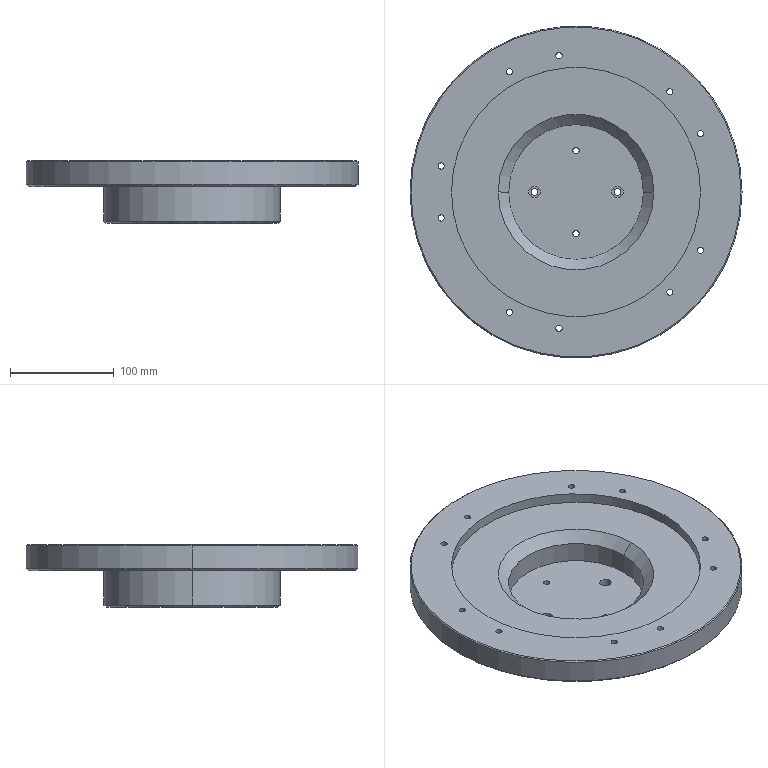NC program | NX | posted with a generic post | part box 320 x 320 x 60 mm
Whole program, first 1569 of 1671 lines:
N10 G17 G21 G94 G90
(FLOOR_WALL_COPY , TOOL : D63)
N12 T01 M6
N14 G54
N16 G17 G0 G90 X-111.041 Y159.693 S6500 M3
N18 G43 Z90. H1
N20 Z63.
N22 G94 G1 Z60. F1250.
N24 X-105.694
N26 X105.696
N28 G2 X107.445 Y158.522 R190.772
N30 X130.313 Y140.326 R191.108
N32 X140.391 Y130.245 R190.747
N34 G1 X-140.394
N36 G3 X-162.829 Y100.796 R191.779
N38 G1 X162.826
N40 G2 X167.72 Y92.43 R190.962
N42 X177.731 Y71.347 R190.522
N44 G1 X-177.72
N46 G3 X-183.779 Y53.845 R190.905
N48 X-186.87 Y41.898 R190.015
N50 G1 X186.872
N52 G2 X188.81 Y32.007 R190.522
N54 X190.35 Y20.971 R189.034
N56 X191.101 Y12.449 R188.892
N58 G1 X-191.099
N60 G3 X-191.307 Y8.671 R190.737
N62 X-191.49 Y2.519 R188.526
N64 G1 Y-2.51
N66 G3 X-191.197 Y-10.802 R188.526
N68 X-190.749 Y-17. R190.562
N70 G1 X190.747
N72 G2 X185.784 Y-46.449 R190.834
N74 G1 X-185.788
N76 G3 X-182.906 Y-56.723 R189.951
N78 X-175.824 Y-75.898 R189.267
N80 G1 X175.831
N82 G2 X159.935 Y-105.347 R190.688
N84 G1 X-159.939
N86 G3 X-151.393 Y-117.272 R184.254
N88 X-136.041 Y-134.796 R190.237
N90 G1 X136.035
N92 X140.226
N94 Z63.
N96 G0 Z90.
N98 M5
(ADAPTIVE_MILLING_COPY , TOOL : D10)
N100 T10 M6
N102 G54
N104 G17 G0 G90 X-167.699 Y-0.751 S7000 M3
N106 G43 Z90. H10
N108 Z45.55
N110 G94 G1 Z42.55 F1000.
N112 X-165.853 Y-0.587 F3000.
N114 G3 X-165.042 Y-0.039 R1.024
N116 X-164.411 Y2.51 R7.406
N118 X-163.825 Y10.487 R163.055
N120 G2 X-150.497 Y65.517 R166.454
N122 X149.112 Y68.574 R164.131
N124 X155.232 Y53.253 R375.404
N126 X5.158 Y-164.038 R164.075
N128 X-164.091 Y-3.174 R164.099
N130 X-163.571 Y2.902 R89.15
N132 X-162.375 Y17.452 R615.566
N134 X148.074 Y68.824 R163.293
N136 X154.541 Y52.674 R266.724
N138 X153.708 Y-55.15 R162.746
N140 X-163.219 Y-4.469 R163.287
N142 X-162.746 Y3.114 R110.67
N144 X-161.065 Y21.334 R295.166
N146 X146.754 Y69.698 R162.464
N148 X154.76 Y49.432 R213.972
N150 X-162.342 Y-6.156 R-162.463
N152 X-161.926 Y3.131 R104.526
N154 X-159.885 Y23.825 R257.116
N156 X145.894 Y69.574 R161.635
N158 X154.348 Y47.983 R200.371
N160 X-161.472 Y-7.049 R-161.633
N162 X-161.066 Y3.739 R119.448
N164 X-158.608 Y26.597 R227.63
N166 X144.775 Y69.997 R160.804
N168 X153.54 Y47.779 R192.297
N170 X-160.584 Y-8.348 R-160.804
N172 X-160.172 Y4.839 R125.799
N174 X-156.919 Y31.22 R200.569
N176 X143.605 Y70.515 R159.979
N178 X153.583 Y44.81 R180.564
N180 X-159.697 Y-9.353 R-159.981
N182 X-159.351 Y4.834 R124.247
N184 X-156. Y31.604 R197.042
N186 X142.382 Y71.125 R159.155
N188 X153.649 Y41.542 R173.736
N190 X-158.796 Y-10.564 R-159.158
N192 X-158.509 Y5.122 R124.27
N194 X-154.853 Y33.058 R191.618
N196 X141.374 Y71.291 R158.324
N198 X152.838 Y41.359 R170.776
N200 X-157.889 Y-11.681 R-158.33
N202 X-157.725 Y4.506 R120.635
N204 X-153.737 Y34.308 R190.113
N206 X140.631 Y70.925 R157.497
N208 X152.312 Y40.119 R168.32
N210 X-156.982 Y-12.703 R-157.502
N212 X-156.891 Y4.682 R121.373
N214 X-152.761 Y34.866 R186.676
N216 X139.478 Y71.367 R156.669
N218 X152.36 Y36.554 R164.249
N220 X-156.122 Y-13.032 R-156.676
N222 X-155.987 Y5.95 R129.61
N224 X-151.223 Y37.751 R179.901
N226 X138.457 Y71.546 R155.842
N228 X151.43 Y36.874 R163.237
N230 X-155.204 Y-14.064 R-155.849
N232 X-155.129 Y6.514 R131.371
N234 X-150.304 Y38.003 R177.491
N236 X137.477 Y71.64 R155.015
N238 X151.366 Y33.5 R160.38
N240 X-154.294 Y-14.9 R-155.021
N242 X-154.34 Y5.976 R128.82
N244 X-149.386 Y38.251 R175.769
N246 X136.122 Y72.443 R154.188
N248 X151.521 Y28.64 R157.78
N250 X-153.369 Y-15.839 R-154.195
N252 X-153.462 Y6.733 R130.459
N254 X-147.931 Y40.526 R171.747
N256 X135.366 Y72.097 R153.359
N258 X151.352 Y24.843 R156.11
N260 X-152.549 Y-15.685 R-153.366
N262 X-152.662 Y6.489 R132.598
N264 X-147.426 Y39.221 R172.911
N266 X133.711 Y73.427 R152.534
N268 X151.266 Y19.744 R154.619
N270 X-151.65 Y-16.329 R-152.538
N272 X-151.81 Y6.841 R133.168
N274 X-146.026 Y41.196 R169.185
N276 X132.568 Y73.784 R151.708
N278 X150.811 Y16.614 R153.419
N280 X16.645 Y-150.815 R151.712
N282 X-150.714 Y-17.27 R151.712
N284 X-150.99 Y6.795 R133.611
N286 X-144.82 Y42.394 R167.722
N288 X132.102 Y72.914 R150.88
N290 X149.799 Y18.15 R152.701
N292 X18.186 Y-149.807 R150.883
N294 X-149.804 Y-17.912 R150.883
N296 X-150.178 Y6.55 R132.106
N298 X-143.829 Y42.822 R165.771
N300 X131.251 Y72.745 R150.053
N302 X149.429 Y13.82 R151.573
N304 X-148.903 Y-18.453 R150.054
N306 X-149.256 Y7.902 R133.377
N308 X-142.307 Y44.972 R163.428
N310 X130.008 Y73.272 R149.224
N312 X148.504 Y14.759 R150.54
N314 X-148.099 Y-18.196 R149.224
N316 X-148.372 Y8.658 R135.611
N318 X-141.051 Y46.159 R161.194
N320 X128.662 Y73.967 R148.394
N322 X148.33 Y4.924 R149.331
N324 X-147.233 Y-18.434 R148.396
N326 X-147.471 Y9.516 R136.787
N328 X-139.127 Y49.235 R157.854
N330 X128.454 Y72.659 R147.566
N332 X147.576 Y1.762 R148.47
N334 X-146.242 Y-19.659 R147.57
N336 X-146.681 Y9.082 R133.855
N338 X-138.561 Y48.342 R157.466
N340 X127.208 Y73.17 R146.734
N342 X146.738 Y-2.405 R147.566
N344 X-145.4 Y-19.687 R146.74
N346 X-145.821 Y9.453 R134.899
N348 X-136.398 Y51.875 R155.266
N350 X126.608 Y72.546 R145.905
N352 X144.722 Y-18.728 R146.401
N354 X-144.547 Y-19.808 R145.909
N356 X-144.88 Y10.726 R136.408
N358 X-134.347 Y54.816 R152.904
N360 X126.012 Y71.916 R145.076
N362 X142.66 Y-26.512 R145.517
N364 X-143.486 Y-21.406 R145.085
N366 X-144.229 Y8.72 R133.432
N368 X-134.283 Y52.745 R153.39
N370 X125.274 Y71.54 R144.251
N372 X144.149 Y-5.85 R144.911
N374 X-142.554 Y-22.003 R144.252
N376 X-143.479 Y7.718 R131.164
N378 X-133.872 Y51.514 R152.99
N380 X124.635 Y70.981 R143.416
N382 X141.417 Y-24.038 R143.816
N384 X-141.637 Y-22.492 R143.424
N386 X-142.69 Y7.225 R131.376
N388 X-132.699 Y52.251 R152.37
N390 X123.308 Y71.628 R142.592
N392 X138.916 Y-32.279 R142.93
N394 X-140.767 Y-22.673 R142.594
N396 X-141.829 Y7.64 R130.576
N398 X-131.097 Y54.014 R150.685
N400 X123.867 Y68.963 R141.762
N402 X58.9 Y-128.979 R141.815
N404 X-139.898 Y-22.842 R141.745
N406 X-140.954 Y8.266 R130.92
N408 X-130.386 Y53.56 R149.841
N410 X135.63 Y38.293 R140.934
N412 X-138.901 Y-23.787 R-140.929
N414 X-140.089 Y8.705 R130.269
N416 X-128.897 Y54.963 R148.15
N418 X121.302 Y70.123 R140.102
N420 X97.155 Y-100.985 R140.198
N422 X-137.931 Y-24.519 R140.096
N424 X-139.254 Y8.761 R129.645
N426 X-127.384 Y56.373 R146.915
N428 X134.78 Y35.088 R139.275
N430 X-136.885 Y-25.627 R-139.269
N432 X-138.549 Y7.139 R127.671
N434 X-126.819 Y55.595 R146.546
N436 X119.752 Y69.49 R138.445
N438 X102.9 Y-92.661 R138.549
N440 X-136.201 Y-24.752 R138.438
N442 X-137.616 Y8.524 R128.789
N444 X-125.679 Y56.112 R145.18
N446 X118.511 Y69.972 R137.618
N448 X121.463 Y-64.745 R137.808
N450 X-135.412 Y-24.45 R137.613
N452 X-136.675 Y9.826 R129.304
N454 X-123.647 Y58.55 R143.55
N456 X117.931 Y69.313 R136.786
N458 X48.497 Y-127.917 R136.813
N460 X-134.588 Y-24.324 R136.745
N462 X-135.831 Y9.952 R128.843
N464 X-122.337 Y59.361 R142.448
N466 X132.864 Y28.822 R135.959
N468 X-133.572 Y-25.259 R-135.947
N470 X-135.064 Y9.202 R127.5
N472 X-121.755 Y58.659 R141.739
N474 X131.4 Y31.491 R135.124
N476 X-132.72 Y-25.288 R-135.115
N478 X-134.275 Y8.674 R126.823
N480 X-121.246 Y57.795 R140.942
N482 X115.856 Y67.919 R134.289
N484 X26.801 Y-131.602 R134.303
N486 X-132.088 Y-24.114 R134.222
N488 X-133.352 Y9.762 R127.509
N490 X-119.639 Y59.202 R139.65
N492 X131.765 Y21.21 R133.468
N494 X-130.954 Y-25.67 R133.453
N496 X-132.589 Y8.981 R126.236
N498 X-119.158 Y58.292 R139.017
N500 X131.636 Y16.232 R132.64
N502 X-130.055 Y-25.922 R132.621
N504 X-131.643 Y10.217 R125.697
N506 X-116.072 Y62.479 R137.001
N508 X130.937 Y15.086 R131.81
N510 X-129.022 Y-26.834 R131.792
N512 X-130.84 Y9.886 R124.887
N514 X-115.395 Y61.976 R136.059
N516 X130.548 Y10.528 R130.976
N518 X-128.172 Y-26.838 R130.96
N520 X-129.972 Y10.278 R124.381
N522 X-114.565 Y61.762 R135.24
N524 X129.689 Y10.818 R130.145
N526 X-127.202 Y-27.4 R130.128
N528 X-129.127 Y10.4 R123.38
N530 X-114.519 Y60.071 R134.471
N532 X110.868 Y66.543 R129.289
N534 X-126.125 Y-28.422 R-129.301
N536 X-128.296 Y10.352 R122.307
N538 X-112.576 Y61.935 R133.333
N540 X109.385 Y67.383 R128.46
N542 X-124.955 Y-29.802 R-128.471
N544 X-127.502 Y9.935 R121.374
N546 X-111.702 Y61.797 R132.559
N548 X126.904 Y13.705 R127.648
N550 X-124.655 Y-27.348 R127.629
N552 X-126.549 Y11.142 R121.707
N554 X-110.664 Y61.946 R131.438
N556 X-86.859 Y-92.405 R-126.816
N558 X-124.847 Y-21.899 R125.96
N560 X-125.312 Y14.565 R123.829
N562 X-105.34 Y69.125 R129.411
N564 X125.656 Y9.031 R125.99
N566 X-122.691 Y-28.486 R125.965
N568 X-124.955 Y10.374 R119.727
N570 X-108.78 Y61.898 R129.761
N572 X124.767 Y9.729 R125.152
N574 X-121.421 Y-30.217 R125.133
N576 X-124.178 Y9.794 R118.71
N578 X-108.621 Y60.482 R129.203
N580 X-96.203 Y-78.746 R-124.318
N582 X-122.555 Y-20.363 R122.928
N584 X-122.585 Y16.101 R122.421
N586 X-99.068 Y73.738 R126.25
N588 X112.961 Y-49.896 R123.496
N590 X-120.048 Y-28.808 R123.465
N592 X-122.326 Y11.527 R118.048
N594 X-105.524 Y62.52 R126.853
N596 X-97.62 Y-74.257 R-122.65
N598 X-121.033 Y-19.257 R121.041
N600 X-120.555 Y18.389 R122.195
N602 X-96.169 Y74.799 R124.293
N604 X107.09 Y58.025 R121.79
N606 X-118.022 Y-30.07 R-121.799
N608 X-120.679 Y11.322 R116.586
N610 X-103.379 Y62.859 R125.301
N612 X120.774 Y7.09 R120.989
N614 X-117.136 Y-30.155 R120.966
N616 X-120.008 Y9.738 R115.469
N618 X-103.66 Y60.763 R124.972
N620 X-93.278 Y-75.734 R-120.149
N622 X-118.217 Y-21.008 R118.896
N624 X-118.303 Y16.632 R118.43
N626 X-94.081 Y73.4 R121.815
N628 X119.035 Y8.088 R119.322
N630 X-115.792 Y-28.651 R119.294
N632 X-118.175 Y11.272 R114.76
N634 X-101.076 Y61.83 R122.839
N636 X103.939 Y56.837 R118.452
N638 X-114.895 Y-28.805 R-118.461
N640 X-117.2 Y12.402 R114.11
N642 X-97.28 Y66.182 R121.253
N644 X106.814 Y49.249 R117.615
N646 X-114.028 Y-28.815 R-117.62
N648 X-116.41 Y11.989 R113.184
N650 X-95.976 Y66.605 R120.37
N652 X103.797 Y53.531 R116.779
N654 X-113.103 Y-29.071 R-116.787
N656 X-115.578 Y11.922 R112.303
N658 X-95.833 Y65.337 R119.566
N660 X-81.851 Y-82.168 R-115.976
N662 X-113.571 Y-23.133 R115.104
N664 X-114.297 Y15.274 R113.391
N666 X-92.904 Y68.036 R118.201
N668 X-80.314 Y-82.505 R-115.14
N670 X-112.728 Y-23.1 R114.301
N672 X-113.201 Y16.886 R113.109
N674 X-91.057 Y69.113 R116.927
N676 X-76.755 Y-84.703 R-114.305
N678 X-111.869 Y-23.114 R113.525
N680 X-112.26 Y17.46 R112.295
N682 X-87.008 Y72.848 R115.55
N684 X-83.119 Y-77.241 R-113.467
N686 X-111.382 Y-21.21 R112.395
N688 X-110.874 Y20.447 R112.816
N690 X-81.695 Y77.548 R114.176
N692 X-73.709 Y-85.167 R-112.632
N694 X-109.942 Y-24.159 R111.895
N696 X-110.915 Y15.314 R110.087
N698 X-89.159 Y67.469 R114.601
N700 X-64.531 Y-91.299 R-111.798
N702 X-108.968 Y-24.696 R111.234
N704 X-110.081 Y15.262 R109.255
N706 X-90.099 Y64.781 R113.906
N708 X110.687 Y7.716 R110.97
N710 X-106.92 Y-29.544 R110.938
N712 X-109.424 Y13.979 R107.582
N714 X-90.271 Y63.089 R113.317
N716 X110.084 Y-2.91 R110.133
N718 X-106.147 Y-29.188 R110.1
N720 X-108.601 Y13.844 R106.889
N722 X-89.081 Y63.322 R112.36
N724 X109.235 Y3.296 R109.295
N726 X-104.989 Y-30.219 R109.264
N728 X-107.917 Y12.678 R105.721
N730 X-88.084 Y63.278 R111.592
N732 X-61.265 Y-89.493 R-108.45
N734 X-105.35 Y-25.485 R107.983
N736 X-106.856 Y14.249 R106.097
N738 X-86.46 Y64.09 R110.587
N740 X-52.586 Y-93.9 R-107.615
N742 X-104.455 Y-25.628 R107.241
N744 X-105.642 Y16.569 R105.729
N746 X-82.974 Y67.209 R109.04
N748 X-59.606 Y-88.598 R-106.774
N750 X-103.665 Y-25.318 R106.349
N752 X-104.618 Y17.567 R105.124
N754 X-79.757 Y69.73 R107.839
N756 X-49.854 Y-93.486 R-105.937
N758 X-102.914 Y-24.846 R105.573
N760 X-103.589 Y18.531 R104.57
N762 X-75.963 Y72.633 R106.656
N764 X-47.1 Y-93.966 R-105.098
N766 X-101.97 Y-25.181 R104.77
N768 X-102.877 Y17.794 R103.577
N770 X-76.461 Y70.882 R105.957
N772 X102.976 Y16.226 R104.26
N774 X-100.524 Y-27.483 R104.228
N776 X-102.304 Y16.239 R102.27
N778 X-78.083 Y67.816 R105.391
N780 X-53.998 Y-88.21 R-103.418
N782 X-100.475 Y-24.186 R102.939
N784 X-101.121 Y18.102 R102.307
N786 X-73.11 Y71.959 R104.195
N788 X-48.01 Y-90.661 R-102.58
N790 X-99.583 Y-24.311 R102.199
N792 X-100.349 Y17.676 R101.415
N794 X-72.075 Y71.811 R103.407
N796 X-55.654 Y-85.176 R-101.739
N798 X-98.886 Y-23.581 R101.192
N800 X-99.215 Y19.092 R100.855
N802 X-62.521 Y79.196 R102.064
N804 X100.87 Y2.216 R100.905
N806 X-96.575 Y-29.065 R100.869
N808 X-99.102 Y15.083 R98.704
N810 X-71.248 Y70.262 R101.899
N812 X-50.538 Y-86.37 R-100.06
N814 X-96.809 Y-25.002 R99.624
N816 X-97.576 Y18.726 R98.775
N818 X-60.892 Y78.338 R100.338
N820 X-53.87 Y-83.328 R-99.217
N822 X-96.107 Y-24.327 R98.682
N824 X-96.326 Y20.573 R98.457
N826 X-51.114 Y84.059 R99.199
N828 X-62.862 Y-75.672 R-98.374
N830 X-95.692 Y-22.4 R97.478
N832 X-95.295 Y21.327 R98.075
N834 X-49.098 Y84.28 R98.323
N836 X-56.725 Y-79.347 R-97.535
N838 X-94.614 Y-23.309 R96.839
N840 X-94.983 Y18.847 R96.598
N842 X-55.952 Y78.865 R97.791
N844 X96.04 Y-11.23 R96.705
N846 X-91.688 Y-30.562 R96.662
N848 X-94.897 Y14.772 R94.242
N850 X-61.287 Y73.707 R97.395
N852 X95.373 Y-9.539 R95.861
N854 X-90.849 Y-30.413 R95.818
N856 X-94.069 Y14.621 R93.509
N858 X-62.509 Y71.559 R96.603
N860 X-63.024 Y-71.09 R-95.006
N862 X-92.705 Y-20.227 R93.851
N864 X-91.427 Y22.974 R95.304
N866 X-42.013 Y84.277 R94.808
N868 X-68.919 Y-64.148 R-94.158
N870 X-92.66 Y-15.754 R92.265
N872 X-84.258 Y40.171 R96.145
N874 X-57.108 Y-73.813 R-93.326
N876 X-90.469 Y-22.474 R92.545
N878 X-90.345 Y20.338 R92.906
N880 X-49.225 Y78.292 R93.383
N882 X-73.322 Y-56.339 R-92.472
N884 X-91.006 Y12.431 R89.768
N886 X-62.032 Y67.458 R93.416
N888 X-64.669 Y-64.906 R-91.63
N890 X-89.879 Y-16.984 R89.903
N892 X-84.765 Y32.634 R92.826
N894 X74.357 Y52.074 R90.82
N896 X-83.379 Y-35.854 R-90.773
N898 X-89.241 Y12.84 R88.343
N900 X-87.005 Y23.41 R128.754
N902 G1 X-85.295 Y29.028
N904 X-85.284 Y29.061
N906 X-83.21 Y34.555
N908 X-83.196 Y34.587
N910 X-80.766 Y39.934
N912 X-80.751 Y39.964
N914 X-77.976 Y45.14
N916 X-77.959 Y45.17
N918 X-74.851 Y50.153
N920 X-74.831 Y50.181
N922 X-71.403 Y54.95
N924 X-71.382 Y54.977
N926 X-67.649 Y59.511
N928 X-67.626 Y59.537
N930 X-63.604 Y63.816
N932 X-63.58 Y63.84
N934 X-59.285 Y67.846
N936 X-59.26 Y67.869
N938 X-54.712 Y71.586
N940 X-54.685 Y71.606
N942 X-49.904 Y75.017
N944 X-49.875 Y75.036
N946 X-44.881 Y78.126
N948 X-44.851 Y78.143
N950 X-39.665 Y80.899
N952 X-39.634 Y80.914
N954 X-34.278 Y83.324
N956 X-34.246 Y83.337
N958 X-28.744 Y85.391
N960 X-28.712 Y85.402
N962 X-23.087 Y87.091
N964 X-23.054 Y87.1
N966 X-17.331 Y88.417
N968 X-17.297 Y88.424
N970 X-11.499 Y89.363
N972 X-11.465 Y89.367
N974 X-5.619 Y89.924
N976 X-5.585 Y89.926
N978 X0.301 Y90.099
N980 X6.189 Y89.887
N982 X6.223 Y89.884
N984 X12.066 Y89.288
N986 X12.1 Y89.283
N988 X17.864 Y88.311
N990 X17.898 Y88.304
N992 X23.586 Y86.958
N994 X23.619 Y86.949
N996 X29.207 Y85.234
N998 X29.24 Y85.223
N1000 X34.704 Y83.148
N1002 X34.736 Y83.134
N1004 X40.054 Y80.707
N1006 X40.084 Y80.692
N1008 X45.232 Y77.923
N1010 X45.262 Y77.905
N1012 X50.219 Y74.806
N1014 X50.247 Y74.787
N1016 X54.991 Y71.372
N1018 X55.018 Y71.351
N1020 X59.529 Y67.633
N1022 X59.554 Y67.61
N1024 X63.813 Y63.606
N1026 X63.837 Y63.582
N1028 X67.826 Y59.309
N1030 X67.849 Y59.283
N1032 X71.55 Y54.759
N1034 X71.571 Y54.732
N1036 X74.969 Y49.975
N1038 X74.988 Y49.947
N1040 X78.069 Y44.979
N1042 X78.086 Y44.95
N1044 X80.837 Y39.791
N1046 X80.852 Y39.761
N1048 X83.26 Y34.434
N1050 X83.273 Y34.403
N1052 X85.328 Y28.93
N1054 X85.339 Y28.898
N1056 X87.034 Y23.303
N1058 X87.043 Y23.27
N1060 X88.368 Y17.577
N1062 X88.375 Y17.544
N1064 X89.327 Y11.776
N1066 X89.331 Y11.742
N1068 X89.904 Y5.925
N1070 X89.907 Y5.891
N1072 X90.1 Y0.031
N1074 X89.928 Y-5.563
N1076 X89.926 Y-5.596
N1078 X89.407 Y-11.152
N1080 X89.403 Y-11.184
N1082 X88.539 Y-16.697
N1084 X88.533 Y-16.729
N1086 X87.327 Y-22.178
N1088 X87.319 Y-22.21
N1090 X85.777 Y-27.573
N1092 X85.767 Y-27.604
N1094 X83.894 Y-32.86
N1096 X83.882 Y-32.891
N1098 X81.685 Y-38.02
N1100 X81.671 Y-38.05
N1102 X79.159 Y-43.033
N1104 X79.143 Y-43.062
N1106 X76.326 Y-47.878
N1108 X76.308 Y-47.906
N1110 X73.034 Y-52.763
N1112 X73.014 Y-52.791
N1114 X69.429 Y-57.424
N1116 X69.408 Y-57.45
N1118 X65.528 Y-61.838
N1120 X65.505 Y-61.863
N1122 X61.347 Y-65.988
N1124 X61.322 Y-66.012
N1126 X56.903 Y-69.856
N1128 X56.877 Y-69.878
N1130 X52.216 Y-73.426
N1132 X52.188 Y-73.446
N1134 X47.306 Y-76.681
N1136 X47.277 Y-76.699
N1138 X42.194 Y-79.609
N1140 X42.164 Y-79.625
N1142 X36.901 Y-82.196
N1144 X36.87 Y-82.21
N1146 X31.451 Y-84.432
N1148 X31.418 Y-84.444
N1150 X25.866 Y-86.307
N1152 X25.833 Y-86.317
N1154 X20.17 Y-87.813
N1156 X20.136 Y-87.82
N1158 X14.388 Y-88.943
N1160 X14.354 Y-88.949
N1162 X8.545 Y-89.693
N1164 X8.511 Y-89.697
N1166 X2.664 Y-90.06
N1168 X2.633 Y-90.061
N1170 X-3.226 Y-90.042
N1172 X-3.261 Y-90.04
N1174 X-9.104 Y-89.638
N1176 X-9.138 Y-89.635
N1178 X-14.943 Y-88.852
N1180 X-14.976 Y-88.846
N1182 X-20.717 Y-87.685
N1184 X-20.751 Y-87.677
N1186 X-26.403 Y-86.144
N1188 X-26.436 Y-86.134
N1190 X-31.977 Y-84.234
N1192 X-32.009 Y-84.222
N1194 X-37.413 Y-81.964
N1196 X-37.444 Y-81.95
N1198 X-42.69 Y-79.344
N1200 X-42.72 Y-79.328
N1202 X-47.784 Y-76.385
N1204 X-47.813 Y-76.367
N1206 X-52.673 Y-73.099
N1208 X-52.701 Y-73.079
N1210 X-57.338 Y-69.5
N1212 X-57.364 Y-69.478
N1214 X-61.757 Y-65.604
N1216 X-61.782 Y-65.581
N1218 X-65.913 Y-61.428
N1220 X-65.936 Y-61.403
N1222 X-69.786 Y-56.989
N1224 X-69.808 Y-56.963
N1226 X-73.361 Y-52.307
N1228 X-73.381 Y-52.279
N1230 X-76.623 Y-47.4
N1232 X-76.641 Y-47.372
N1234 G2 X-81.879 Y-37.6 R105.305
N1236 X-85.878 Y-27.257 R105.312
N1238 X-88.575 Y-16.502 R105.312
N1240 X-89.932 Y-5.497 R105.312
N1242 G1 X-90.1 Y0.03
N1244 X-89.905 Y5.918
N1246 X-89.903 Y5.952
N1248 X-89.324 Y11.797
N1250 X-89.319 Y11.831
N1252 X-88.359 Y17.625
N1254 X-88.352 Y17.658
N1256 X-87.418 Y21.65
N1258 G3 X-88.324 Y22.888 R1.014
N1260 G1 X-89.672 Y22.991
N1262 Z45.55
N1264 G0 Z90.
N1266 X-92.795 Y0.
N1268 Z62.003
N1270 G1 Z59.003 F1000.
N1272 X-91.324 Y-0.459 F3000.
N1274 G3 X-90.148 Y0. R1.017
N1276 X-89.437 Y2.526 R6.856
N1278 G2 X-88.361 Y12.065 R374.925
N1280 X-71.52 Y-53.258 R-89.171
N1282 X-75.508 Y-47.372 R593.008
N1284 X-80.018 Y-39.357 R120.656
N1286 X-89.105 Y-2.561 R87.818
N1288 G3 X-89.138 Y-0.02 R38.159
N1290 G1 X-88.948 Y5.819
N1292 X-88.946 Y5.853
N1294 X-88.373 Y11.65
N1296 X-88.369 Y11.684
N1298 X-87.417 Y17.43
N1300 X-87.411 Y17.464
N1302 X-86.083 Y23.135
N1304 X-86.074 Y23.168
N1306 X-84.378 Y28.74
N1308 X-84.367 Y28.773
N1310 X-82.307 Y34.221
N1312 X-82.294 Y34.253
N1314 X-79.882 Y39.554
N1316 X-79.866 Y39.585
N1318 X-77.111 Y44.716
N1320 X-77.093 Y44.746
N1322 X-74.007 Y49.685
N1324 X-73.987 Y49.714
N1326 X-70.583 Y54.439
N1328 X-70.562 Y54.467
N1330 X-66.854 Y58.959
N1332 X-66.831 Y58.984
N1334 X-62.837 Y63.223
N1336 X-62.812 Y63.247
N1338 X-58.548 Y67.214
N1340 X-58.522 Y67.237
N1342 X-54.006 Y70.915
N1344 X-53.978 Y70.936
N1346 X-49.23 Y74.31
N1348 X-49.202 Y74.329
N1350 X-44.243 Y77.383
N1352 X-44.213 Y77.4
N1354 X-39.063 Y80.123
N1356 X-39.032 Y80.138
N1358 X-33.716 Y82.516
N1360 X-33.684 Y82.529
N1362 X-28.222 Y84.552
N1364 X-28.189 Y84.563
N1366 X-22.607 Y86.224
N1368 X-22.573 Y86.232
N1370 X-16.894 Y87.522
N1372 X-16.86 Y87.529
N1374 X-11.108 Y88.443
N1376 X-11.073 Y88.448
N1378 X-5.274 Y88.982
N1380 X-5.239 Y88.984
N1382 X0.594 Y89.136
N1384 X6.437 Y88.905
N1386 X6.472 Y88.903
N1388 X12.264 Y88.29
N1390 X12.298 Y88.286
N1392 X17.984 Y87.305
N1394 X18.018 Y87.298
N1396 X23.628 Y85.949
N1398 X23.661 Y85.94
N1400 X29.172 Y84.229
N1402 X29.204 Y84.218
N1404 X34.591 Y82.152
N1406 X34.623 Y82.139
N1408 X39.865 Y79.727
N1410 X39.895 Y79.712
N1412 X44.969 Y76.964
N1414 X44.998 Y76.946
N1416 X49.882 Y73.874
N1418 X49.911 Y73.855
N1420 X54.584 Y70.471
N1422 X54.611 Y70.45
N1424 X59.055 Y66.769
N1426 X59.081 Y66.746
N1428 X63.275 Y62.784
N1430 X63.299 Y62.76
N1432 X67.227 Y58.533
N1434 X67.25 Y58.507
N1436 X70.894 Y54.033
N1438 X70.915 Y54.006
N1440 X74.26 Y49.305
N1442 X74.279 Y49.277
N1444 X77.312 Y44.368
N1446 X77.329 Y44.338
N1448 X80.035 Y39.242
N1450 X80.05 Y39.211
N1452 X82.42 Y33.95
N1454 X82.433 Y33.918
N1456 X84.454 Y28.514
N1458 X84.465 Y28.482
N1460 X86.131 Y22.957
N1462 X86.14 Y22.924
N1464 X87.442 Y17.303
N1466 X87.449 Y17.269
N1468 X88.383 Y11.575
N1470 X88.388 Y11.542
N1472 X88.949 Y5.799
N1474 X88.951 Y5.765
N1476 X89.138 Y-0.02
N1478 X88.965 Y-5.549
N1480 X88.963 Y-5.581
N1482 X88.448 Y-11.073
N1484 X88.444 Y-11.105
N1486 X87.587 Y-16.554
N1488 X87.581 Y-16.586
N1490 X86.388 Y-21.971
N1492 X86.38 Y-22.002
N1494 X84.854 Y-27.303
N1496 X84.844 Y-27.334
N1498 X82.991 Y-32.529
N1500 X82.979 Y-32.559
N1502 X80.806 Y-37.629
N1504 X80.793 Y-37.658
N1506 X78.309 Y-42.583
N1508 X78.293 Y-42.612
N1510 X75.508 Y-47.372
N1512 X75.49 Y-47.4
N1514 X72.262 Y-52.189
N1516 X72.242 Y-52.217
N1518 X68.71 Y-56.785
N1520 X68.688 Y-56.812
N1522 X64.865 Y-61.14
N1524 X64.842 Y-61.165
N1526 X60.745 Y-65.235
N1528 X60.72 Y-65.259
N1530 X56.367 Y-69.053
N1532 X56.34 Y-69.075
N1534 X51.749 Y-72.578
N1536 X51.722 Y-72.598
N1538 X46.912 Y-75.795
N1540 X46.883 Y-75.813
N1542 X41.876 Y-78.689
N1544 X41.846 Y-78.705
N1546 X36.661 Y-81.25
N1548 X36.63 Y-81.264
N1550 X31.291 Y-83.465
N1552 X31.259 Y-83.477
N1554 X25.788 Y-85.326
N1556 X25.756 Y-85.336
N1558 X20.176 Y-86.825
N1560 X20.143 Y-86.832
N1562 X14.478 Y-87.954
N1564 X14.444 Y-87.96
N1566 X8.718 Y-88.711
N1568 X8.684 Y-88.714
N1570 X2.922 Y-89.09
N1572 X2.887 Y-89.091
N1574 X-2.887
N1576 X-2.922 Y-89.09
N1578 X-8.684 Y-88.714
N1580 X-8.718 Y-88.711
N1582 X-14.444 Y-87.96
N1584 X-14.478 Y-87.954
N1586 X-20.143 Y-86.832
N1588 X-20.176 Y-86.825
N1590 X-25.756 Y-85.336
N1592 X-25.788 Y-85.326
N1594 X-31.259 Y-83.477
N1596 X-31.291 Y-83.465
N1598 X-36.63 Y-81.264
N1600 X-36.661 Y-81.25
N1602 X-41.846 Y-78.705
N1604 X-41.876 Y-78.689
N1606 X-46.883 Y-75.813
N1608 X-46.912 Y-75.795
N1610 X-51.722 Y-72.598
N1612 X-51.749 Y-72.578
N1614 X-56.34 Y-69.075
N1616 X-56.367 Y-69.053
N1618 X-60.72 Y-65.259
N1620 X-60.745 Y-65.235
N1622 X-64.842 Y-61.165
N1624 X-64.865 Y-61.14
N1626 X-68.688 Y-56.812
N1628 X-68.71 Y-56.785
N1630 X-72.242 Y-52.217
N1632 X-72.262 Y-52.189
N1634 X-75.49 Y-47.4
N1636 X-75.508 Y-47.372
N1638 X-78.293 Y-42.612
N1640 X-78.309 Y-42.583
N1642 X-80.793 Y-37.658
N1644 X-80.806 Y-37.629
N1646 X-82.979 Y-32.559
N1648 X-82.991 Y-32.529
N1650 X-84.844 Y-27.334
N1652 X-84.854 Y-27.303
N1654 X-86.38 Y-22.002
N1656 X-86.388 Y-21.971
N1658 X-87.581 Y-16.586
N1660 X-87.587 Y-16.554
N1662 X-88.444 Y-11.105
N1664 X-88.448 Y-11.073
N1666 X-88.963 Y-5.581
N1668 X-88.965 Y-5.549
N1670 X-89.078 Y-1.95
N1672 G3 X-90.126 Y-0.973 R1.014
N1674 G1 X-91.457 Y-1.024
N1676 Z62.003
N1678 G0 Z90.
N1680 X-167.7 Y-0.752
N1682 Z28.1
N1684 G1 Z25.1 F1000.
N1686 X-165.854 Y-0.588 F3000.
N1688 G3 X-165.044 Y-0.04 R1.024
N1690 X-164.412 Y2.509 R7.403
N1692 X-163.827 Y10.486 R162.42
N1694 G2 X-152.859 Y59.783 R166.573
N1696 X149.23 Y68.305 R164.119
N1698 X155.166 Y53.448 R410.848
N1700 X-88.126 Y-138.453 R164.103
N1702 X-164.092 Y-3.082 R164.037
N1704 X-163.508 Y3.591 R121.795
N1706 X-162.069 Y20.025 R304.249
N1708 X148.233 Y68.47 R163.282
N1710 X154.672 Y52.309 R260.699
N1712 X61.143 Y-151.418 R163.202
N1714 X-163.223 Y-4.486 R163.274
N1716 X-162.676 Y4.095 R148.592
N1718 X-160.561 Y24.881 R247.607
N1720 X147.205 Y68.718 R162.453
N1722 X154.377 Y50.591 R222.805
N1724 X-162.347 Y-6.084 R-162.46
N1726 X-161.96 Y2.704 R103.55
N1728 X-159.876 Y23.896 R260.095
N1730 X145.964 Y69.42 R161.635
N1732 X154.312 Y48.11 R200.655
N1734 X-161.47 Y-7.188 R-161.636
N1736 X-161.01 Y4.599 R127.931
N1738 X-158.478 Y27.347 R215.632
N1740 X144.841 Y69.853 R160.802
N1742 X153.504 Y47.917 R192.042
N1744 X-160.59 Y-8.297 R-160.809
N1746 X-160.23 Y3.992 R119.696
N1748 X-157.252 Y29.502 R209.569
N1750 X143.449 Y70.831 R159.982
N1752 X153.457 Y45.246 R180.558
N1754 X-159.713 Y-9.114 R-159.983
N1756 X-159.305 Y5.572 R129.984
N1758 X-155.833 Y32.426 R194.499
N1760 X142.659 Y70.552 R159.149
N1762 X153.011 Y43.819 R175.213
N1764 X-158.819 Y-10.238 R-159.158
N1766 X-158.495 Y5.449 R130.394
N1768 X-155.034 Y32.203 R193.738
N1770 X141.473 Y71.091 R158.327
N1772 X153.059 Y40.566 R170.705
N1774 X-157.92 Y-11.268 R-158.334
N1776 X-157.67 Y5.518 R131.532
N1778 X-153.819 Y33.931 R189.514
N1780 X140.321 Y71.541 R157.504
N1782 X152.546 Y39.238 R167.313
N1784 X-157.051 Y-11.804 R-157.504
N1786 X-156.848 Y5.482 R132.678
N1788 X-152.673 Y35.257 R185.868
N1790 X139.067 Y72.169 R156.675
N1792 X152.39 Y36.46 R163.976
N1794 X-156.169 Y-12.443 R-156.679
N1796 X-155.951 Y6.639 R135.158
N1798 X-151.762 Y35.505 R181.537
N1800 X138.543 Y71.378 R155.84
N1802 X151.712 Y35.72 R162.27
N1804 X-155.246 Y-13.587 R-155.852
N1806 X-155.164 Y6.095 R131.411
N1808 X-150.67 Y36.527 R179.505
N1810 X137.468 Y71.659 R155.016
N1812 X151.792 Y31.569 R159.718
N1814 X-154.303 Y-14.833 R-155.028
N1816 X-154.344 Y6.044 R130.68
N1818 X-149.17 Y39.091 R176.325
N1820 X136.573 Y71.589 R154.191
N1822 X151.652 Y27.989 R157.808
N1824 X-153.299 Y-16.58 R-154.204
N1826 X-153.493 Y6.389 R130.3
N1828 X-148.096 Y39.902 R172.595
N1830 X135.346 Y72.139 R153.361
N1832 X151.184 Y25.877 R156.164
N1834 X-152.447 Y-16.738 R-153.374
N1836 X-152.663 Y6.429 R130.176
N1838 X-146.36 Y43.015 R169.183
N1840 X134.159 Y72.6 R152.529
N1842 X150.726 Y23.567 R155.048
N1844 X-151.539 Y-17.395 R-152.546
N1846 X-151.864 Y6.071 R130.207
N1848 X-145.932 Y41.51 R169.421
N1850 X133.204 Y72.621 R151.7
N1852 X150.086 Y22.243 R153.78
N1854 X-150.571 Y-18.55 R-151.718
N1856 X-151.04 Y6.008 R129.542
N1858 X-144.731 Y42.692 R167.689
N1860 X132.963 Y71.325 R150.874
N1862 X149.041 Y23.59 R153.076
N1864 X-149.615 Y-19.506 R-150.889
N1866 X-150.194 Y6.344 R130.112
N1868 X-143.453 Y44.06 R165.526
N1870 X131.583 Y72.14 R150.049
N1872 X148.732 Y19.991 R151.835
N1874 X20.019 Y-148.741 R150.063
N1876 X-148.572 Y-21.054 R150.063
N1878 X-149.379 Y6.184 R129.584
N1880 X-142.812 Y43.325 R164.8
N1882 X130.674 Y72.07 R149.215
N1884 X148.127 Y18.166 R150.632
N1886 X-147.752 Y-20.913 R149.23
N1888 X-148.51 Y6.824 R130.899
N1890 X-141.906 Y43.452 R163.188
N1892 X129.673 Y72.174 R148.39
N1894 X148.035 Y10.559 R149.488
N1896 X-146.792 Y-21.759 R148.403
N1898 X-147.728 Y6.171 R129.922
N1900 X-141.119 Y43.201 R162.978
N1902 X128.326 Y72.882 R147.563
N1904 X147.553 Y2.921 R148.313
N1906 X-145.96 Y-21.71 R147.572
N1908 X-146.827 Y7.218 R130.499
N1910 X-140.062 Y43.814 R161.074
N1912 X127.912 Y71.929 R146.735
N1914 X146.631 Y-6.129 R147.415
N1916 X-144.859 Y-23.432 R146.748
N1918 X-145.98 Y7.474 R130.501
N1920 X-138.966 Y44.527 R159.448
N1922 X127.691 Y70.616 R145.904
N1924 X145.477 Y-11.479 R146.439
N1926 X-143.866 Y-24.355 R145.918
N1928 X-145.201 Y6.84 R130.083
N1930 X-137.391 Y46.669 R158.337
N1932 X126.259 Y71.483 R145.078
N1934 X142.648 Y-26.608 R145.528
N1936 X-142.85 Y-25.368 R145.094
N1938 X-144.388 Y6.613 R129.435
N1940 X-136.335 Y47.2 R157.043
N1942 X125.317 Y71.469 R144.256
N1944 X141.248 Y-29.427 R144.714
N1946 X-142.019 Y-25.287 R144.263
N1948 X-143.543 Y6.892 R129.404
N1950 X-134.934 Y48.679 R155.564
N1952 X124.128 Y71.88 R143.433
N1954 X143.237 Y-7.613 R144.031
N1956 X-141.395 Y-24.016 R143.427
N1958 X-142.611 Y8.278 R130.736
N1960 X-132.973 Y51.56 R152.638
N1962 X124.425 Y69.672 R142.596
N1964 X129.312 Y-60.17 R142.836
N1966 X-140.209 Y-25.984 R142.605
N1968 X-141.728 Y8.877 R130.079
N1970 X-131.197 Y53.776 R150.427
N1972 X123.3 Y69.977 R141.765
N1974 X115.976 Y-81.579 R141.88
N1976 X-139.199 Y-26.853 R141.774
N1978 X-140.905 Y8.792 R129.195
N1980 X-130.488 Y53.309 R149.483
N1982 X135.476 Y38.847 R140.937
N1984 X-138.524 Y-25.937 R-140.935
N1986 X-140.076 Y8.822 R129.303
N1988 X-129.818 Y52.766 R149.255
N1990 X136.214 Y32.814 R140.118
N1992 X-137.483 Y-26.974 R-140.108
N1994 X-139.229 Y9.065 R129.109
N1996 X-128.647 Y53.438 R148.263
N1998 X135.3 Y33.053 R139.286
N2000 X-136.57 Y-27.307 R-139.277
N2002 X-138.418 Y8.825 R128.383
N2004 X-127.886 Y53.106 R147.301
N2006 X119.996 Y69.067 R138.45
N2008 X-134.903 Y-31.142 R-138.453
N2010 X-137.572 Y9. R127.775
N2012 X-125.855 Y55.73 R145.323
N2014 X137.553 Y-4.378 R137.632
N2016 X-135.194 Y-25.662 R137.612
N2018 X-136.61 Y10.49 R129.048
N2020 X-124.377 Y56.98 R143.609
N2022 X117.25 Y70.46 R136.781
N2024 X-134.068 Y-27.118 R-136.79
N2026 X-135.783 Y10.406 R128.01
N2028 X-123.675 Y56.517 R142.554
N2030 X135.157 Y14.761 R135.966
N2032 X-133.306 Y-26.69 R135.955
N2034 X-134.931 Y10.64 R127.807
N2036 X-123.087 Y55.798 R141.695
N2038 X-129.292 Y-39.336 R-135.14
N2040 X-134.16 Y9.999 R126.279
N2042 X-122.287 Y55.556 R141.031
N2044 X-127.511 Y-42.208 R-134.31
N2046 X-133.32 Y10.078 R125.781
N2048 X-120.931 Y56.514 R139.644
N2050 X-110.37 Y-75.076 R-133.479
N2052 X-132.186 Y-17.861 R131.456
N2054 X-131.876 Y15.548 R131.74
N2056 X-112.46 Y70.356 R135.9
N2058 X-107.928 Y-77.126 R-132.649
N2060 X-131.297 Y-18.228 R130.751
N2062 X-131.075 Y15.279 R130.727
N2064 X-111.172 Y70.841 R135.105
N2066 X35.839 Y-126.848 R-131.818
N2068 X-128.627 Y-28.711 R131.768
N2070 X-130.811 Y10.165 R124.065
N2072 X-117.017 Y58.853 R136.2
N2074 X-125.2 Y-38.49 R-130.982
N2076 X-129.998 Y9.948 R123.085
N2078 X-115.655 Y59.701 R135.361
N2080 X-123.669 Y-40.57 R-130.151
N2082 X-129.193 Y9.661 R122.5
N2084 X-115.501 Y58.166 R134.575
N2086 X-123.023 Y-39.856 R-129.317
N2088 X-128.27 Y10.597 R122.046
N2090 X-113.078 Y61.009 R133.071
N2092 X-122.863 Y-37.588 R-128.484
N2094 X-127.495 Y9.97 R121.097
N2096 X-113.566 Y58.297 R132.601
N2098 X-122.053 Y-37.388 R-127.652
N2100 X-126.662 Y9.972 R120.388
N2102 X-113.008 Y57.556 R131.79
N2104 X-121.514 Y-36.296 R-126.818
N2106 X-125.737 Y10.902 R120.088
N2108 X-110.338 Y60.826 R130.675
N2110 X-120.199 Y-37.753 R-125.988
N2112 X-124.86 Y11.269 R119.51
N2114 X-108.532 Y62.33 R129.261
N2116 X-119.265 Y-37.932 R-125.153
N2118 X-124.026 Y11.273 R118.789
N2120 X-106.629 Y63.933 R128.331
N2122 X-108.939 Y-59.901 R-124.321
N2124 X-123.489 Y-12.747 R120.326
N2126 X-120.096 Y28.93 R128.733
N2128 X100.56 Y71.686 R123.542
N2130 X37.934 Y-117.531 R123.53
N2132 X-119.834 Y-29.723 R123.48
N2134 X-122.243 Y12.282 R118.237
N2136 X-104.931 Y63.515 R126.447
N2138 X-116.438 Y-38.545 R-122.653
N2140 X-121.45 Y11.9 R116.843
N2142 X-105.055 Y61.683 R125.884
N2144 X-113.941 Y-43.101 R-121.82
N2146 X-120.706 Y11.06 R115.932
N2148 X-104.488 Y61. R125.253
N2150 X16.762 Y-119.812 R-120.986
N2152 X-117.69 Y-27.896 R120.866
N2154 X-119.627 Y13.142 R116.464
N2156 X-101.834 Y63.777 R123.737
N2158 X-113.578 Y-39.191 R-120.151
N2160 X-118.974 Y11.591 R114.69
N2162 X-102.43 Y61.205 R123.41
N2164 X-110.39 Y-45.277 R-119.316
N2166 X-118.302 Y10.081 R113.747
N2168 X-102.908 Y58.731 R123.105
N2170 X-108.845 Y-46.803 R-118.482
N2172 X-117.376 Y10.903 R113.16
N2174 X-101.401 Y59.666 R121.998
N2176 X-109.015 Y-44.227 R-117.646
N2178 X-116.472 Y11.472 R112.395
N2180 X-98.369 Y63.005 R120.384
N2182 X-109.681 Y-40.184 R-116.811
N2184 X-115.559 Y12.088 R111.795
N2186 X-96.464 Y64.392 R119.199
N2188 X105.961 Y47.088 R115.937
N2190 X-111.975 Y-30.098 R-115.954
N2192 X-114.6 Y13.048 R111.905
N2194 X-93.516 Y67.184 R118.062
N2196 X110.306 Y-33.03 R115.148
N2198 X-110.716 Y-31.52 R115.125
N2200 X-113.847 Y12.373 R110.756
N2202 X-94.81 Y63.853 R117.392
N2204 X-107.889 Y-37.741 R-114.302
N2206 X-113.178 Y10.955 R109.61
N2208 X-95.13 Y61.859 R117.017
N2210 X109.931 Y-28.147 R113.478
N2212 X-109.435 Y-29.874 R113.452
N2214 X-112.29 Y11.377 R109.536
N2216 X-94.589 Y61.157 R116.066
N2218 X109.81 Y-25.084 R112.641
N2220 X-108.161 Y-31.332 R112.62
N2222 X-111.464 Y11.259 R108.617
N2224 X-92.076 Y63.414 R115.073
N2226 X-94.067 Y-60.412 R-111.795
N2228 X-110.775 Y-13.651 R108.529
N2230 X-94.946 Y57.433 R115.101
N2232 X-83.66 Y-72.893 R-110.959
N2234 X-109.072 Y-19.794 R109.372
N2236 X-108.224 Y20.965 R111.145
N2238 X-64.592 Y89.193 R111.077
N2240 X-86.939 Y-67.591 R-110.122
N2242 X-108.653 Y-17.072 R107.982
N2244 X-105.903 Y27.248 R112.13
N2246 X-1.456 Y109.282 R109.509
N2248 X-61.243 Y-90.522 R-109.29
N2250 X-106.207 Y-25.504 R108.741
N2252 X-107.443 Y15.914 R107.176
N2254 X-79.629 Y73.622 R110.269
N2256 X-101.477 Y-38.241 R-108.445
N2258 X-107.373 Y10.243 R104.409
N2260 X-88.458 Y61.288 R110.834
N2262 X-99.152 Y-41.813 R-107.609
N2264 X-106.604 Y9.586 R103.434
N2266 X-88.307 Y60.024 R110.158
N2268 X-84.118 Y-65.756 R-106.771
N2270 X-105.093 Y-18.121 R104.668
N2272 X-103.351 Y23.677 R107.829
N2274 X-40.409 Y97.932 R106.496
N2276 X-78.512 Y-71.119 R-105.935
N2278 X-103.784 Y-20.707 R104.399
N2280 X-102.815 Y22.283 R106.056
N2282 X-51.715 Y91.495 R105.833
N2284 X-97.338 Y-39.621 R-105.094
N2286 X-103.854 Y11.492 R101.354
N2288 X-79.948 Y66.92 R106.711
N2290 X-82.416 Y-63.846 R-104.255
N2292 X-102.756 Y-16.705 R101.853
N2294 X-99.475 Y28.524 R106.198
N2296 X8.012 Y103.115 R103.619
N2298 X-56.119 Y-86.87 R-103.422
N2300 X-100.523 Y-23.986 R102.779
N2302 X-100.768 Y19.873 R102.752
N2304 X-62.474 Y81.36 R103.695
N2306 X-94.731 Y-39.332 R-102.575
N2308 X-101.437 Y10.559 R99.008
N2310 X-77.037 Y66.458 R104.177
N2312 X-80.439 Y-62.285 R-101.736
N2314 X-100.056 Y-17.606 R99.324
N2316 X-97.739 Y25.412 R103.04
N2318 X-22.646 Y98.332 R101.332
N2320 X-77.368 Y-64.763 R-100.898
N2322 X-99.158 Y-17.887 R98.858
N2324 X-96.045 Y28.305 R102.479
N2326 X-2.906 Y100.025 R100.324
N2328 X-85.144 Y-52.546 R-100.056
N2330 X-98.908 Y10.506 R96.609
N2332 X-75.034 Y64.915 R101.474
N2334 X-91.315 Y-38.778 R-99.213
N2336 X-97.802 Y12.467 R95.919
N2338 X-68.441 Y70.671 R100.199
N2340 X-82.052 Y-54.265 R-98.375
N2342 X-96.944 Y12.53 R95.201
N2344 X-65.419 Y72.347 R99.202
N2346 X-81.436 Y-53.667 R-97.532
N2348 X-96.215 Y11.69 R94.411
N2350 X-65.992 Y70.679 R98.498
N2352 X-85.398 Y-45.333 R-96.689
N2354 X-95.493 Y10.742 R93.46
N2356 X-68.117 Y67.437 R97.816
N2358 X-86.802 Y-40.62 R-95.846
N2360 X-94.467 Y12.065 R92.845
N2362 X-65.671 Y68.663 R96.832
N2364 X-84.979 Y-42.459 R-95.003
N2366 X-93.71 Y11.402 R91.956
N2368 X-64.935 Y68.2 R96.038
N2370 X-84.197 Y-42.139 R-94.161
N2372 X-92.816 Y11.728 R91.274
N2374 X-63.982 Y67.94 R95.156
N2376 X-83.813 Y-41.012 R-93.317
N2378 X-91.757 Y13.139 R90.574
N2380 X-61.326 Y69.224 R94.143
N2382 X-83.291 Y-40.15 R-92.473
N2384 X-90.884 Y13.266 R89.833
N2386 X-61.332 Y68.089 R93.333
N2388 X-81.85 Y-41.171 R-91.63
N2390 X-90.21 Y12.113 R88.971
N2392 X-62.858 Y65.514 R92.675
N2394 X-82.293 Y-38.317 R-90.784
N2396 X-89.242 Y12.848 R88.339
N2398 X-87.005 Y23.41 R129.575
N2400 G1 X-85.295 Y29.028
N2402 X-85.284 Y29.061
N2404 X-83.21 Y34.555
N2406 X-83.196 Y34.587
N2408 X-80.766 Y39.934
N2410 X-80.751 Y39.964
N2412 X-77.976 Y45.14
N2414 X-77.959 Y45.17
N2416 X-74.851 Y50.153
N2418 X-74.831 Y50.181
N2420 X-71.403 Y54.95
N2422 X-71.382 Y54.977
N2424 X-67.649 Y59.511
N2426 X-67.626 Y59.537
N2428 X-63.604 Y63.816
N2430 X-63.58 Y63.84
N2432 X-59.285 Y67.846
N2434 X-59.26 Y67.869
N2436 X-54.712 Y71.586
N2438 X-54.685 Y71.606
N2440 X-49.904 Y75.017
N2442 X-49.875 Y75.036
N2444 X-44.881 Y78.126
N2446 X-44.851 Y78.143
N2448 X-39.665 Y80.899
N2450 X-39.634 Y80.914
N2452 X-34.278 Y83.324
N2454 X-34.246 Y83.337
N2456 X-28.744 Y85.391
N2458 X-28.712 Y85.402
N2460 X-23.087 Y87.091
N2462 X-23.054 Y87.1
N2464 X-17.331 Y88.417
N2466 X-17.297 Y88.424
N2468 X-11.499 Y89.363
N2470 X-11.465 Y89.367
N2472 X-5.619 Y89.924
N2474 X-5.585 Y89.926
N2476 X0.301 Y90.099
N2478 X6.189 Y89.887
N2480 X6.223 Y89.884
N2482 X12.066 Y89.288
N2484 X12.1 Y89.283
N2486 X17.864 Y88.311
N2488 X17.898 Y88.304
N2490 X23.586 Y86.958
N2492 X23.619 Y86.949
N2494 X29.207 Y85.234
N2496 X29.24 Y85.223
N2498 X34.704 Y83.148
N2500 X34.736 Y83.134
N2502 X40.054 Y80.707
N2504 X40.084 Y80.692
N2506 X45.232 Y77.923
N2508 X45.262 Y77.905
N2510 X50.219 Y74.806
N2512 X50.247 Y74.787
N2514 X54.991 Y71.372
N2516 X55.018 Y71.351
N2518 X59.529 Y67.633
N2520 X59.554 Y67.61
N2522 X63.813 Y63.606
N2524 X63.837 Y63.582
N2526 X67.826 Y59.309
N2528 X67.849 Y59.283
N2530 X71.55 Y54.759
N2532 X71.571 Y54.732
N2534 X74.969 Y49.975
N2536 X74.988 Y49.947
N2538 X78.069 Y44.979
N2540 X78.086 Y44.95
N2542 X80.837 Y39.791
N2544 X80.852 Y39.761
N2546 X83.26 Y34.434
N2548 X83.273 Y34.403
N2550 X85.328 Y28.93
N2552 X85.339 Y28.898
N2554 X87.034 Y23.303
N2556 X87.043 Y23.27
N2558 X88.368 Y17.577
N2560 X88.375 Y17.544
N2562 X89.327 Y11.776
N2564 X89.331 Y11.742
N2566 X89.904 Y5.925
N2568 X89.907 Y5.891
N2570 X90.1 Y0.031
N2572 X89.928 Y-5.563
N2574 X89.926 Y-5.596
N2576 X89.407 Y-11.152
N2578 X89.403 Y-11.184
N2580 X88.539 Y-16.697
N2582 X88.533 Y-16.729
N2584 X87.327 Y-22.178
N2586 X87.319 Y-22.21
N2588 X85.777 Y-27.573
N2590 X85.767 Y-27.604
N2592 X83.894 Y-32.86
N2594 X83.882 Y-32.891
N2596 X81.685 Y-38.02
N2598 X81.671 Y-38.05
N2600 X79.159 Y-43.033
N2602 X79.143 Y-43.062
N2604 X76.326 Y-47.878
N2606 X76.308 Y-47.906
N2608 X73.034 Y-52.763
N2610 X73.014 Y-52.791
N2612 X69.429 Y-57.424
N2614 X69.408 Y-57.45
N2616 X65.528 Y-61.838
N2618 X65.505 Y-61.863
N2620 X61.347 Y-65.988
N2622 X61.322 Y-66.012
N2624 X56.903 Y-69.856
N2626 X56.877 Y-69.878
N2628 X52.216 Y-73.426
N2630 X52.188 Y-73.446
N2632 X47.306 Y-76.681
N2634 X47.277 Y-76.699
N2636 X42.194 Y-79.609
N2638 X42.164 Y-79.625
N2640 X36.901 Y-82.196
N2642 X36.87 Y-82.21
N2644 X31.451 Y-84.432
N2646 X31.418 Y-84.444
N2648 X25.866 Y-86.307
N2650 X25.833 Y-86.317
N2652 X20.17 Y-87.813
N2654 X20.136 Y-87.82
N2656 X14.388 Y-88.943
N2658 X14.354 Y-88.949
N2660 X8.545 Y-89.693
N2662 X8.511 Y-89.697
N2664 X2.664 Y-90.06
N2666 X2.633 Y-90.061
N2668 X-3.226 Y-90.042
N2670 X-3.261 Y-90.04
N2672 X-9.104 Y-89.638
N2674 X-9.138 Y-89.635
N2676 X-14.943 Y-88.852
N2678 X-14.976 Y-88.846
N2680 X-20.717 Y-87.685
N2682 X-20.751 Y-87.677
N2684 X-26.403 Y-86.144
N2686 X-26.436 Y-86.134
N2688 X-31.977 Y-84.234
N2690 X-32.009 Y-84.222
N2692 X-37.413 Y-81.964
N2694 X-37.444 Y-81.95
N2696 X-42.69 Y-79.344
N2698 X-42.72 Y-79.328
N2700 X-47.784 Y-76.385
N2702 X-47.813 Y-76.367
N2704 X-52.673 Y-73.099
N2706 X-52.701 Y-73.079
N2708 X-57.338 Y-69.5
N2710 X-57.364 Y-69.478
N2712 X-61.757 Y-65.604
N2714 X-61.782 Y-65.581
N2716 X-65.913 Y-61.428
N2718 X-65.936 Y-61.403
N2720 X-69.786 Y-56.989
N2722 X-69.808 Y-56.963
N2724 X-73.361 Y-52.307
N2726 X-73.381 Y-52.279
N2728 X-76.623 Y-47.4
N2730 X-76.641 Y-47.372
N2732 G2 X-81.879 Y-37.6 R105.305
N2734 X-85.878 Y-27.257 R105.312
N2736 X-88.575 Y-16.502 R105.312
N2738 X-89.932 Y-5.497 R105.312
N2740 G1 X-90.1 Y0.03
N2742 X-89.905 Y5.918
N2744 X-89.903 Y5.952
N2746 X-89.324 Y11.797
N2748 X-89.319 Y11.831
N2750 X-88.359 Y17.625
N2752 X-88.352 Y17.658
N2754 X-87.418 Y21.65
N2756 G3 X-88.324 Y22.888 R1.014
N2758 G1 X-89.672 Y22.991
N2760 Z28.1
N2762 G0 Z90.
N2764 M5
(FLOOR_WALL_1_COPY_1_COPY , TOOL : D10JING)
N2766 T11 M6
N2768 G54
N2770 G17 G0 G90 X-1.658 Y164.492 S7000 M3
N2772 G43 Z90. H11
N2774 Z26.5
N2776 G94 G1 Z25. F1000.
N2778 X-1.086 Y163.5
N2780 G3 X-0.22 Y163. R1.
N2782 G1 X0.216
N2784 G2 X39.876 Y158.047 R163.
N2786 G1 X-39.879 Y158.046
N2788 G3 X-55.96 Y153.093 R163.
N2790 G1 X55.957 Y153.094
N2792 G2 X67.994 Y148.141 R163.
N2794 G1 X-67.997 Y148.14
N2796 G3 X-77.889 Y143.187 R163.
N2798 G1 X77.885 Y143.188
N2800 G2 X86.371 Y138.235 R163.
N2802 G1 X-86.375 Y138.233
N2804 G3 X-93.837 Y133.28 R163.
N2806 G1 X93.834 Y133.282
N2808 G2 X100.502 Y128.329 R163.
N2810 G1 X-100.505 Y128.327
N2812 G3 X-106.527 Y123.374 R163.
N2814 G1 X106.524 Y123.376
N2816 G2 X112.004 Y118.423 R163.
N2818 G1 X-112.007 Y118.421
N2820 G3 X-117.022 Y113.467 R163.
N2822 G1 X117.02 Y113.47
N2824 G2 X121.627 Y108.517 R163.
N2826 G1 X-121.629 Y108.514
N2828 G3 X-125.873 Y103.561 R163.
N2830 G1 X125.871 Y103.564
N2832 G2 X129.788 Y98.611 R163.
N2834 G1 X-129.79 Y98.608
N2836 G3 X-133.408 Y93.655 R163.
N2838 G1 X133.406 Y93.658
N2840 G2 X136.75 Y88.705 R163.
N2842 G1 X18.442 Y88.703
N2844 G2 X34.558 Y83.75 R90.6
N2846 G1 X139.838 Y83.751
N2848 G2 X142.688 Y78.798 R163.
N2850 G1 X44.714 Y78.797
N2852 G2 X52.492 Y73.844 R90.6
N2854 G1 X145.313 Y73.845
N2856 G2 X147.726 Y68.892 R163.
N2858 G1 X58.842 Y68.891
N2860 G2 X64.189 Y63.938 R90.6
N2862 G1 X149.936 Y63.939
N2864 G2 X151.953 Y58.986 R163.
N2866 G1 X68.769 Y58.985
N2868 G2 X72.725 Y54.032 R90.6
N2870 G1 X153.784 Y54.033
N2872 G2 X155.435 Y49.08 R163.
N2874 G1 X76.155 Y49.079
N2876 G2 X79.128 Y44.126 R90.6
N2878 G1 X156.913 Y44.127
N2880 G2 X158.223 Y39.174 R163.
N2882 G1 X81.694 Y39.173
N2884 G2 X83.889 Y34.22 R90.6
N2886 G1 X159.367
N2888 G2 X160.351 Y29.267 R163.
N2890 G1 X85.743
N2892 G2 X87.277 Y24.313 R90.6
N2894 G1 X161.176 Y24.314
N2896 G2 X161.846 Y19.361 R163.
N2898 G1 X88.507 Y19.36
N2900 G2 X89.447 Y14.407 R90.6
N2902 G1 X162.362 Y14.408
N2904 G2 X162.726 Y9.455 R163.
N2906 G1 X90.105 Y9.454
N2908 G2 X90.488 Y4.501 R90.6
N2910 G1 X162.938 Y4.502
N2912 G2 X162.999 Y-0.451 R163.
N2914 G1 X90.599 Y-0.452
N2916 G2 X90.439 Y-5.405 R90.6
N2918 G1 X162.91 Y-5.404
N2920 G2 X162.671 Y-10.358 R163.
N2922 G1 X90.006
N2924 G2 X89.297 Y-15.311 R90.6
N2926 G1 X162.279
N2928 G2 X161.736 Y-20.264 R163.
N2930 G1 X88.305 Y-20.265
N2932 G2 X87.02 Y-25.218 R90.6
N2934 G1 X161.038 Y-25.217
N2936 G2 X160.184 Y-30.17 R163.
N2938 G1 X85.429 Y-30.171
N2940 G2 X83.514 Y-35.124 R90.6
N2942 G1 X159.171 Y-35.123
N2944 G2 X157.996 Y-40.076 R163.
N2946 G1 X81.254 Y-40.077
N2948 G2 X78.617 Y-45.03 R90.6
N2950 G1 X156.657 Y-45.029
N2952 G2 X155.147 Y-49.983 R163.
N2954 G1 X75.565
N2956 G2 X72.044 Y-54.937 R90.6
N2958 G1 X153.464 Y-54.936
N2960 G2 X151.599 Y-59.889 R163.
N2962 G1 X67.982 Y-59.89
N2964 G2 X63.275 Y-64.843 R90.6
N2966 G1 X149.548 Y-64.842
N2968 G2 X147.301 Y-69.795 R163.
N2970 G1 X57.766 Y-69.796
N2972 G2 X51.195 Y-74.749 R90.6
N2974 G1 X144.851 Y-74.748
N2976 G2 X142.185 Y-79.701 R163.
N2978 G1 X43.08 Y-79.703
N2980 G2 X32.276 Y-84.656 R90.6
N2982 G1 X139.293 Y-84.655
N2984 G2 X136.16 Y-89.608 R163.
N2986 G1 X13.363 Y-89.609
N2988 Z26.5
N2990 G0 Z90.
N2992 X18.442 Y88.703
N2994 Z26.5
N2996 G1 Z25.
N2998 G3 X-18.444 Y88.703 R90.6
N3000 G1 X-136.752 Y88.702
N3002 G3 X-139.84 Y83.748 R163.
N3004 G1 X-34.56 Y83.75
N3006 G3 X-44.716 Y78.796 R90.6
N3008 G1 X-142.69 Y78.795
N3010 G3 X-145.315 Y73.842 R163.
N3012 G1 X-52.493 Y73.843
N3014 G3 X-58.843 Y68.89 R90.6
N3016 G1 X-147.727 Y68.889
N3018 G3 X-149.937 Y63.936 R163.
N3020 G1 X-64.191 Y63.937
N3022 G3 X-68.77 Y58.984 R90.6
N3024 G1 X-151.954 Y58.983
N3026 G3 X-153.785 Y54.03 R163.
N3028 G1 X-72.726
N3030 G3 X-76.156 Y49.077 R90.6
N3032 G1 X-155.437 Y49.076
N3034 G3 X-156.914 Y44.123 R163.
N3036 G1 X-79.129 Y44.124
N3038 G3 X-81.695 Y39.171 R90.6
N3040 G1 X-158.224 Y39.17
N3042 G3 X-159.368 Y34.217 R163.
N3044 G1 X-83.89 Y34.218
N3046 G3 X-85.743 Y29.265 R90.6
N3048 G1 X-160.352 Y29.264
N3050 G3 X-161.177 Y24.311 R163.
N3052 G1 X-87.277 Y24.312
N3054 G3 X-88.508 Y19.358 R90.6
N3056 G1 X-161.846
N3058 G3 X-162.362 Y14.404 R163.
N3060 G1 X-89.447 Y14.405
N3062 G3 X-90.106 Y9.452 R90.6
N3064 G1 X-162.726 Y9.451
N3066 G3 X-162.938 Y4.498 R163.
N3068 G1 X-90.488 Y4.499
N3070 G3 X-90.599 Y-0.454 R90.6
N3072 G1 X-162.999 Y-0.455
N3074 G3 X-162.91 Y-5.408 R163.
N3076 G1 X-90.438 Y-5.407
N3078 G3 X-90.006 Y-10.36 R90.6
N3080 G1 X-162.67 Y-10.361
N3082 G3 X-162.279 Y-15.314 R163.
N3084 G1 X-89.296 Y-15.313
N3086 G3 X-88.304 Y-20.267 R90.6
N3088 G1 X-161.735
N3090 G3 X-161.037 Y-25.221 R163.
N3092 G1 X-87.019 Y-25.22
N3094 G3 X-85.428 Y-30.173 R90.6
N3096 G1 X-160.183 Y-30.174
N3098 G3 X-159.17 Y-35.127 R163.
N3100 G1 X-83.514 Y-35.126
N3102 G3 X-81.253 Y-40.079 R90.6
N3104 G1 X-157.996 Y-40.08
N3106 G3 X-156.656 Y-45.033 R163.
N3108 G1 X-78.616 Y-45.032
N3110 G3 X-75.564 Y-49.985 R90.6
N3112 G1 X-155.146 Y-49.986
N3114 G3 X-153.462 Y-54.939 R163.
N3116 G1 X-72.043 Y-54.938
N3118 G3 X-67.981 Y-59.891 R90.6
N3120 G1 X-151.598 Y-59.892
N3122 G3 X-149.546 Y-64.845 R163.
N3124 G1 X-63.274 Y-64.844
N3126 G3 X-57.764 Y-69.797 R90.6
N3128 G1 X-147.3 Y-69.798
N3130 G3 X-144.849 Y-74.752 R163.
N3132 G1 X-51.193 Y-74.75
N3134 G3 X-43.078 Y-79.704 R90.6
N3136 G1 X-142.184 Y-79.705
N3138 G3 X-139.291 Y-84.658 R163.
N3140 G1 X-32.274 Y-84.657